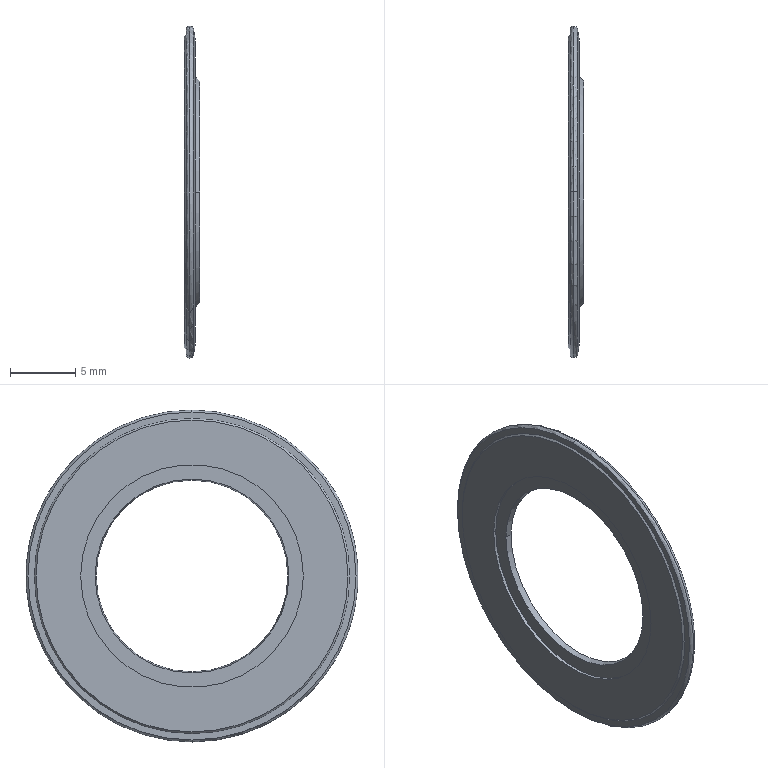Part | SolidWorks | features BaseBody 1 | 1 solid | 23 faces | box 1.155 x 25.353 x 25.353 mm | volume 179.548 mm3 | cone 8 | cylinder 6 | plane 5 | torus 4 | commonest cylinder face diameters 17 x4 23.324 x2
STEP:
#1=CARTESIAN_POINT('',(0.456,0.,12.676));
#2=VERTEX_POINT('',#1);
#3=CARTESIAN_POINT('',(0.456,0.,-12.676));
#4=VERTEX_POINT('',#3);
#5=CARTESIAN_POINT('',(0.456,0.,0.));
#6=DIRECTION('',(1.,0.,0.));
#7=DIRECTION('',(0.,0.,-1.));
#8=AXIS2_PLACEMENT_3D('',#5,#6,#7);
#9=CIRCLE('',#8,12.676);
#10=EDGE_CURVE('',#2,#4,#9,.T.);
#11=ORIENTED_EDGE('',*,*,#10,.T.);
#12=CARTESIAN_POINT('',(0.7554,0.,-12.425));
#13=VERTEX_POINT('',#12);
#14=CARTESIAN_POINT('',(0.456,0.,-12.372));
#15=DIRECTION('',(0.,-1.,0.));
#16=DIRECTION('',(0.,0.,-1.));
#17=AXIS2_PLACEMENT_3D('',#14,#15,#16);
#18=CIRCLE('',#17,0.304);
#19=EDGE_CURVE('',#4,#13,#18,.T.);
#20=ORIENTED_EDGE('',*,*,#19,.T.);
#21=CARTESIAN_POINT('',(0.7554,-12.425,0.));
#22=VERTEX_POINT('',#21);
#23=CARTESIAN_POINT('',(0.7554,0.,0.));
#24=DIRECTION('',(1.,0.,0.));
#25=DIRECTION('',(0.,1.,0.));
#26=AXIS2_PLACEMENT_3D('',#23,#24,#25);
#27=CIRCLE('',#26,12.425);
#28=EDGE_CURVE('',#22,#13,#27,.T.);
#29=ORIENTED_EDGE('',*,*,#28,.F.);
#30=CARTESIAN_POINT('',(0.7554,0.,12.425));
#31=VERTEX_POINT('',#30);
#32=CARTESIAN_POINT('',(0.7554,0.,0.));
#33=DIRECTION('',(1.,0.,0.));
#34=DIRECTION('',(0.,1.,0.));
#35=AXIS2_PLACEMENT_3D('',#32,#33,#34);
#36=CIRCLE('',#35,12.425);
#37=EDGE_CURVE('',#31,#22,#36,.T.);
#38=ORIENTED_EDGE('',*,*,#37,.F.);
#39=CARTESIAN_POINT('',(0.456,0.,12.372));
#40=DIRECTION('',(0.,-1.,0.));
#41=DIRECTION('',(0.,0.,1.));
#42=AXIS2_PLACEMENT_3D('',#39,#40,#41);
#43=CIRCLE('',#42,0.304);
#44=EDGE_CURVE('',#31,#2,#43,.T.);
#45=ORIENTED_EDGE('',*,*,#44,.T.);
#46=EDGE_LOOP('',(#11,#20,#29,#38,#45));
#47=FACE_OUTER_BOUND('',#46,.T.);
#48=CARTESIAN_POINT('',(0.456,0.,0.));
#49=DIRECTION('',(1.,0.,0.));
#50=DIRECTION('',(0.,0.,-1.));
#51=AXIS2_PLACEMENT_3D('',#48,#49,#50);
#52=TOROIDAL_SURFACE('',#51,12.372,0.304);
#53=ADVANCED_FACE('',(#47),#52,.T.);
#54=CARTESIAN_POINT('',(0.1927,12.038,0.));
#55=VERTEX_POINT('',#54);
#56=CARTESIAN_POINT('',(0.1927,-12.038,0.));
#57=VERTEX_POINT('',#56);
#58=CARTESIAN_POINT('',(0.1927,0.,0.));
#59=DIRECTION('',(1.,0.,0.));
#60=DIRECTION('',(0.,1.,0.));
#61=AXIS2_PLACEMENT_3D('',#58,#59,#60);
#62=CIRCLE('',#61,12.038);
#63=EDGE_CURVE('',#55,#57,#62,.T.);
#64=ORIENTED_EDGE('',*,*,#63,.T.);
#65=CARTESIAN_POINT('',(0.1927,0.,0.));
#66=DIRECTION('',(1.,0.,0.));
#67=DIRECTION('',(0.,1.,0.));
#68=AXIS2_PLACEMENT_3D('',#65,#66,#67);
#69=CIRCLE('',#68,12.038);
#70=EDGE_CURVE('',#57,#55,#69,.T.);
#71=ORIENTED_EDGE('',*,*,#70,.T.);
#72=EDGE_LOOP('',(#64,#71));
#73=FACE_BOUND('',#72,.T.);
#74=CARTESIAN_POINT('',(0.1927,0.,-12.524));
#75=VERTEX_POINT('',#74);
#76=CARTESIAN_POINT('',(0.1927,0.,12.524));
#77=VERTEX_POINT('',#76);
#78=CARTESIAN_POINT('',(0.1927,0.,0.));
#79=DIRECTION('',(1.,0.,0.));
#80=DIRECTION('',(0.,1.,0.));
#81=AXIS2_PLACEMENT_3D('',#78,#79,#80);
#82=CIRCLE('',#81,12.524);
#83=EDGE_CURVE('',#75,#77,#82,.T.);
#84=ORIENTED_EDGE('',*,*,#83,.F.);
#85=CARTESIAN_POINT('',(0.1927,0.,0.));
#86=DIRECTION('',(1.,0.,0.));
#87=DIRECTION('',(0.,1.,0.));
#88=AXIS2_PLACEMENT_3D('',#85,#86,#87);
#89=CIRCLE('',#88,12.524);
#90=EDGE_CURVE('',#77,#75,#89,.T.);
#91=ORIENTED_EDGE('',*,*,#90,.F.);
#92=EDGE_LOOP('',(#84,#91));
#93=FACE_OUTER_BOUND('',#92,.T.);
#94=CARTESIAN_POINT('',(0.1927,12.281,0.));
#95=DIRECTION('',(-1.,0.,0.));
#96=DIRECTION('',(0.,1.,0.));
#97=AXIS2_PLACEMENT_3D('',#94,#95,#96);
#98=PLANE('',#97);
#99=ADVANCED_FACE('',(#73,#93),#98,.T.);
#100=CARTESIAN_POINT('',(0.0608,11.906,0.));
#101=VERTEX_POINT('',#100);
#102=CARTESIAN_POINT('',(0.1268,11.972,0.));
#103=DIRECTION('',(0.7071,0.7071,0.));
#104=VECTOR('',#103,1000.);
#105=LINE('',#102,#104);
#106=EDGE_CURVE('',#101,#55,#105,.T.);
#107=ORIENTED_EDGE('',*,*,#106,.T.);
#108=ORIENTED_EDGE('',*,*,#70,.F.);
#109=CARTESIAN_POINT('',(0.0608,-11.906,0.));
#110=VERTEX_POINT('',#109);
#111=CARTESIAN_POINT('',(0.1268,-11.972,0.));
#112=DIRECTION('',(-0.7071,0.7071,0.));
#113=VECTOR('',#112,1000.);
#114=LINE('',#111,#113);
#115=EDGE_CURVE('',#57,#110,#114,.T.);
#116=ORIENTED_EDGE('',*,*,#115,.T.);
#117=CARTESIAN_POINT('',(0.0608,0.,0.));
#118=DIRECTION('',(1.,0.,0.));
#119=DIRECTION('',(0.,1.,0.));
#120=AXIS2_PLACEMENT_3D('',#117,#118,#119);
#121=CIRCLE('',#120,11.906);
#122=EDGE_CURVE('',#110,#101,#121,.T.);
#123=ORIENTED_EDGE('',*,*,#122,.T.);
#124=EDGE_LOOP('',(#107,#108,#116,#123));
#125=FACE_OUTER_BOUND('',#124,.T.);
#126=CARTESIAN_POINT('',(0.1268,0.,0.));
#127=DIRECTION('',(1.,0.,0.));
#128=DIRECTION('',(0.,1.,0.));
#129=AXIS2_PLACEMENT_3D('',#126,#127,#128);
#130=CONICAL_SURFACE('',#129,11.972,0.7854);
#131=ADVANCED_FACE('',(#125),#130,.T.);
#132=CARTESIAN_POINT('',(0.0608,8.5,0.));
#133=VERTEX_POINT('',#132);
#134=CARTESIAN_POINT('',(0.0608,-8.5,0.));
#135=VERTEX_POINT('',#134);
#136=CARTESIAN_POINT('',(0.0608,0.,0.));
#137=DIRECTION('',(1.,0.,0.));
#138=DIRECTION('',(0.,1.,0.));
#139=AXIS2_PLACEMENT_3D('',#136,#137,#138);
#140=CIRCLE('',#139,8.5);
#141=EDGE_CURVE('',#133,#135,#140,.T.);
#142=ORIENTED_EDGE('',*,*,#141,.T.);
#143=CARTESIAN_POINT('',(0.0608,0.,0.));
#144=DIRECTION('',(1.,0.,0.));
#145=DIRECTION('',(0.,1.,0.));
#146=AXIS2_PLACEMENT_3D('',#143,#144,#145);
#147=CIRCLE('',#146,8.5);
#148=EDGE_CURVE('',#135,#133,#147,.T.);
#149=ORIENTED_EDGE('',*,*,#148,.T.);
#150=EDGE_LOOP('',(#142,#149));
#151=FACE_BOUND('',#150,.T.);
#152=CARTESIAN_POINT('',(0.0608,0.,0.));
#153=DIRECTION('',(1.,0.,0.));
#154=DIRECTION('',(0.,1.,0.));
#155=AXIS2_PLACEMENT_3D('',#152,#153,#154);
#156=CIRCLE('',#155,11.906);
#157=EDGE_CURVE('',#101,#110,#156,.T.);
#158=ORIENTED_EDGE('',*,*,#157,.F.);
#159=ORIENTED_EDGE('',*,*,#122,.F.);
#160=EDGE_LOOP('',(#158,#159));
#161=FACE_OUTER_BOUND('',#160,.T.);
#162=CARTESIAN_POINT('',(0.0608,10.203,0.));
#163=DIRECTION('',(-1.,0.,0.));
#164=DIRECTION('',(0.,0.,1.));
#165=AXIS2_PLACEMENT_3D('',#162,#163,#164);
#166=PLANE('',#165);
#167=ADVANCED_FACE('',(#151,#161),#166,.T.);
#168=CARTESIAN_POINT('',(0.2888,8.5,0.));
#169=VERTEX_POINT('',#168);
#170=CARTESIAN_POINT('',(0.1748,8.5,0.));
#171=DIRECTION('',(1.,0.,0.));
#172=VECTOR('',#171,1000.);
#173=LINE('',#170,#172);
#174=EDGE_CURVE('',#133,#169,#173,.T.);
#175=ORIENTED_EDGE('',*,*,#174,.T.);
#176=CARTESIAN_POINT('',(0.2888,-8.5,0.));
#177=VERTEX_POINT('',#176);
#178=CARTESIAN_POINT('',(0.2888,0.,0.));
#179=DIRECTION('',(1.,0.,0.));
#180=DIRECTION('',(0.,1.,0.));
#181=AXIS2_PLACEMENT_3D('',#178,#179,#180);
#182=CIRCLE('',#181,8.5);
#183=EDGE_CURVE('',#169,#177,#182,.T.);
#184=ORIENTED_EDGE('',*,*,#183,.T.);
#185=CARTESIAN_POINT('',(0.1748,-8.5,0.));
#186=DIRECTION('',(-1.,0.,0.));
#187=VECTOR('',#186,1000.);
#188=LINE('',#185,#187);
#189=EDGE_CURVE('',#177,#135,#188,.T.);
#190=ORIENTED_EDGE('',*,*,#189,.T.);
#191=ORIENTED_EDGE('',*,*,#141,.F.);
#192=EDGE_LOOP('',(#175,#184,#190,#191));
#193=FACE_OUTER_BOUND('',#192,.T.);
#194=CARTESIAN_POINT('',(0.1748,0.,0.));
#195=DIRECTION('',(1.,0.,0.));
#196=DIRECTION('',(0.,1.,0.));
#197=AXIS2_PLACEMENT_3D('',#194,#195,#196);
#198=CYLINDRICAL_SURFACE('',#197,8.5);
#199=ADVANCED_FACE('',(#193),#198,.F.);
#200=CARTESIAN_POINT('',(0.2888,7.405,0.));
#201=VERTEX_POINT('',#200);
#202=CARTESIAN_POINT('',(0.2888,-7.405,0.));
#203=VERTEX_POINT('',#202);
#204=CARTESIAN_POINT('',(0.2888,0.,0.));
#205=DIRECTION('',(1.,0.,0.));
#206=DIRECTION('',(0.,1.,0.));
#207=AXIS2_PLACEMENT_3D('',#204,#205,#206);
#208=CIRCLE('',#207,7.405);
#209=EDGE_CURVE('',#201,#203,#208,.T.);
#210=ORIENTED_EDGE('',*,*,#209,.T.);
#211=CARTESIAN_POINT('',(0.2888,0.,0.));
#212=DIRECTION('',(1.,0.,0.));
#213=DIRECTION('',(0.,1.,0.));
#214=AXIS2_PLACEMENT_3D('',#211,#212,#213);
#215=CIRCLE('',#214,7.405);
#216=EDGE_CURVE('',#203,#201,#215,.T.);
#217=ORIENTED_EDGE('',*,*,#216,.T.);
#218=EDGE_LOOP('',(#210,#217));
#219=FACE_BOUND('',#218,.T.);
#220=ORIENTED_EDGE('',*,*,#183,.F.);
#221=CARTESIAN_POINT('',(0.2888,0.,0.));
#222=DIRECTION('',(1.,0.,0.));
#223=DIRECTION('',(0.,1.,0.));
#224=AXIS2_PLACEMENT_3D('',#221,#222,#223);
#225=CIRCLE('',#224,8.5);
#226=EDGE_CURVE('',#177,#169,#225,.T.);
#227=ORIENTED_EDGE('',*,*,#226,.F.);
#228=EDGE_LOOP('',(#220,#227));
#229=FACE_OUTER_BOUND('',#228,.T.);
#230=CARTESIAN_POINT('',(0.2888,7.953,0.));
#231=DIRECTION('',(-1.,0.,0.));
#232=DIRECTION('',(0.,1.,0.));
#233=AXIS2_PLACEMENT_3D('',#230,#231,#232);
#234=PLANE('',#233);
#235=ADVANCED_FACE('',(#219,#229),#234,.T.);
#236=CARTESIAN_POINT('',(0.76,7.322,0.));
#237=VERTEX_POINT('',#236);
#238=CARTESIAN_POINT('',(0.5244,7.364,0.));
#239=DIRECTION('',(0.9848,-0.1736,0.));
#240=VECTOR('',#239,1000.);
#241=LINE('',#238,#240);
#242=EDGE_CURVE('',#201,#237,#241,.T.);
#243=ORIENTED_EDGE('',*,*,#242,.T.);
#244=CARTESIAN_POINT('',(0.76,-7.322,0.));
#245=VERTEX_POINT('',#244);
#246=CARTESIAN_POINT('',(0.76,0.,0.));
#247=DIRECTION('',(1.,0.,0.));
#248=DIRECTION('',(0.,1.,0.));
#249=AXIS2_PLACEMENT_3D('',#246,#247,#248);
#250=CIRCLE('',#249,7.322);
#251=EDGE_CURVE('',#237,#245,#250,.T.);
#252=ORIENTED_EDGE('',*,*,#251,.T.);
#253=CARTESIAN_POINT('',(0.5244,-7.364,0.));
#254=DIRECTION('',(-0.9848,-0.1736,0.));
#255=VECTOR('',#254,1000.);
#256=LINE('',#253,#255);
#257=EDGE_CURVE('',#245,#203,#256,.T.);
#258=ORIENTED_EDGE('',*,*,#257,.T.);
#259=ORIENTED_EDGE('',*,*,#209,.F.);
#260=EDGE_LOOP('',(#243,#252,#258,#259));
#261=FACE_OUTER_BOUND('',#260,.T.);
#262=CARTESIAN_POINT('',(0.5244,0.,0.));
#263=DIRECTION('',(-1.,0.,0.));
#264=DIRECTION('',(0.,1.,0.));
#265=AXIS2_PLACEMENT_3D('',#262,#263,#264);
#266=CONICAL_SURFACE('',#265,7.364,0.1745);
#267=ADVANCED_FACE('',(#261),#266,.F.);
#268=ORIENTED_EDGE('',*,*,#251,.F.);
#269=CARTESIAN_POINT('',(0.76,0.,0.));
#270=DIRECTION('',(1.,0.,0.));
#271=DIRECTION('',(0.,1.,0.));
#272=AXIS2_PLACEMENT_3D('',#269,#270,#271);
#273=CIRCLE('',#272,7.322);
#274=EDGE_CURVE('',#245,#237,#273,.T.);
#275=ORIENTED_EDGE('',*,*,#274,.F.);
#276=EDGE_LOOP('',(#268,#275));
#277=FACE_BOUND('',#276,.T.);
#278=CARTESIAN_POINT('',(0.76,8.5,0.));
#279=VERTEX_POINT('',#278);
#280=CARTESIAN_POINT('',(0.76,-8.5,0.));
#281=VERTEX_POINT('',#280);
#282=CARTESIAN_POINT('',(0.76,0.,0.));
#283=DIRECTION('',(1.,0.,0.));
#284=DIRECTION('',(0.,1.,0.));
#285=AXIS2_PLACEMENT_3D('',#282,#283,#284);
#286=CIRCLE('',#285,8.5);
#287=EDGE_CURVE('',#279,#281,#286,.T.);
#288=ORIENTED_EDGE('',*,*,#287,.T.);
#289=CARTESIAN_POINT('',(0.76,0.,0.));
#290=DIRECTION('',(1.,0.,0.));
#291=DIRECTION('',(0.,1.,0.));
#292=AXIS2_PLACEMENT_3D('',#289,#290,#291);
#293=CIRCLE('',#292,8.5);
#294=EDGE_CURVE('',#281,#279,#293,.T.);
#295=ORIENTED_EDGE('',*,*,#294,.T.);
#296=EDGE_LOOP('',(#288,#295));
#297=FACE_OUTER_BOUND('',#296,.T.);
#298=CARTESIAN_POINT('',(0.76,7.911,0.));
#299=DIRECTION('',(1.,0.,0.));
#300=DIRECTION('',(0.,1.,0.));
#301=AXIS2_PLACEMENT_3D('',#298,#299,#300);
#302=PLANE('',#301);
#303=ADVANCED_FACE('',(#277,#297),#302,.T.);
#304=CARTESIAN_POINT('',(1.216,8.5,0.));
#305=VERTEX_POINT('',#304);
#306=CARTESIAN_POINT('',(0.988,8.5,0.));
#307=DIRECTION('',(1.,0.,0.));
#308=VECTOR('',#307,1000.);
#309=LINE('',#306,#308);
#310=EDGE_CURVE('',#279,#305,#309,.T.);
#311=ORIENTED_EDGE('',*,*,#310,.T.);
#312=CARTESIAN_POINT('',(1.216,-8.5,0.));
#313=VERTEX_POINT('',#312);
#314=CARTESIAN_POINT('',(1.216,0.,0.));
#315=DIRECTION('',(1.,0.,0.));
#316=DIRECTION('',(0.,1.,0.));
#317=AXIS2_PLACEMENT_3D('',#314,#315,#316);
#318=CIRCLE('',#317,8.5);
#319=EDGE_CURVE('',#305,#313,#318,.T.);
#320=ORIENTED_EDGE('',*,*,#319,.T.);
#321=CARTESIAN_POINT('',(0.988,-8.5,0.));
#322=DIRECTION('',(-1.,0.,0.));
#323=VECTOR('',#322,1000.);
#324=LINE('',#321,#323);
#325=EDGE_CURVE('',#313,#281,#324,.T.);
#326=ORIENTED_EDGE('',*,*,#325,.T.);
#327=ORIENTED_EDGE('',*,*,#287,.F.);
#328=EDGE_LOOP('',(#311,#320,#326,#327));
#329=FACE_OUTER_BOUND('',#328,.T.);
#330=CARTESIAN_POINT('',(0.988,0.,0.));
#331=DIRECTION('',(1.,0.,0.));
#332=DIRECTION('',(0.,1.,0.));
#333=AXIS2_PLACEMENT_3D('',#330,#331,#332);
#334=CYLINDRICAL_SURFACE('',#333,8.5);
#335=ADVANCED_FACE('',(#329),#334,.F.);
#336=CARTESIAN_POINT('',(0.5168,9.199,0.));
#337=VERTEX_POINT('',#336);
#338=CARTESIAN_POINT('',(0.8664,8.85,0.));
#339=DIRECTION('',(0.7071,-0.7071,0.));
#340=VECTOR('',#339,1000.);
#341=LINE('',#338,#340);
#342=EDGE_CURVE('',#337,#305,#341,.T.);
#343=ORIENTED_EDGE('',*,*,#342,.T.);
#344=CARTESIAN_POINT('',(1.216,0.,0.));
#345=DIRECTION('',(1.,0.,0.));
#346=DIRECTION('',(0.,1.,0.));
#347=AXIS2_PLACEMENT_3D('',#344,#345,#346);
#348=CIRCLE('',#347,8.5);
#349=EDGE_CURVE('',#313,#305,#348,.T.);
#350=ORIENTED_EDGE('',*,*,#349,.F.);
#351=CARTESIAN_POINT('',(0.5168,-9.199,0.));
#352=VERTEX_POINT('',#351);
#353=CARTESIAN_POINT('',(0.8664,-8.85,0.));
#354=DIRECTION('',(-0.7071,-0.7071,0.));
#355=VECTOR('',#354,1000.);
#356=LINE('',#353,#355);
#357=EDGE_CURVE('',#313,#352,#356,.T.);
#358=ORIENTED_EDGE('',*,*,#357,.T.);
#359=CARTESIAN_POINT('',(0.5168,0.,0.));
#360=DIRECTION('',(1.,0.,0.));
#361=DIRECTION('',(0.,1.,0.));
#362=AXIS2_PLACEMENT_3D('',#359,#360,#361);
#363=CIRCLE('',#362,9.199);
#364=EDGE_CURVE('',#352,#337,#363,.T.);
#365=ORIENTED_EDGE('',*,*,#364,.T.);
#366=EDGE_LOOP('',(#343,#350,#358,#365));
#367=FACE_OUTER_BOUND('',#366,.T.);
#368=CARTESIAN_POINT('',(0.8664,0.,0.));
#369=DIRECTION('',(-1.,0.,0.));
#370=DIRECTION('',(0.,1.,0.));
#371=AXIS2_PLACEMENT_3D('',#368,#369,#370);
#372=CONICAL_SURFACE('',#371,8.85,0.7854);
#373=ADVANCED_FACE('',(#367),#372,.T.);
#374=CARTESIAN_POINT('',(0.5168,0.,0.));
#375=DIRECTION('',(1.,0.,0.));
#376=DIRECTION('',(0.,1.,0.));
#377=AXIS2_PLACEMENT_3D('',#374,#375,#376);
#378=CIRCLE('',#377,9.199);
#379=EDGE_CURVE('',#337,#352,#378,.T.);
#380=ORIENTED_EDGE('',*,*,#379,.F.);
#381=ORIENTED_EDGE('',*,*,#364,.F.);
#382=EDGE_LOOP('',(#380,#381));
#383=FACE_BOUND('',#382,.T.);
#384=CARTESIAN_POINT('',(0.5168,11.662,0.));
#385=VERTEX_POINT('',#384);
#386=CARTESIAN_POINT('',(0.5168,-11.662,0.));
#387=VERTEX_POINT('',#386);
#388=CARTESIAN_POINT('',(0.5168,0.,0.));
#389=DIRECTION('',(1.,0.,0.));
#390=DIRECTION('',(0.,1.,0.));
#391=AXIS2_PLACEMENT_3D('',#388,#389,#390);
#392=CIRCLE('',#391,11.662);
#393=EDGE_CURVE('',#385,#387,#392,.T.);
#394=ORIENTED_EDGE('',*,*,#393,.T.);
#395=CARTESIAN_POINT('',(0.5168,0.,0.));
#396=DIRECTION('',(1.,0.,0.));
#397=DIRECTION('',(0.,1.,0.));
#398=AXIS2_PLACEMENT_3D('',#395,#396,#397);
#399=CIRCLE('',#398,11.662);
#400=EDGE_CURVE('',#387,#385,#399,.T.);
#401=ORIENTED_EDGE('',*,*,#400,.T.);
#402=EDGE_LOOP('',(#394,#401));
#403=FACE_OUTER_BOUND('',#402,.T.);
#404=CARTESIAN_POINT('',(0.5168,10.431,0.));
#405=DIRECTION('',(1.,0.,0.));
#406=DIRECTION('',(0.,1.,0.));
#407=AXIS2_PLACEMENT_3D('',#404,#405,#406);
#408=PLANE('',#407);
#409=ADVANCED_FACE('',(#383,#403),#408,.T.);
#410=CARTESIAN_POINT('',(0.8899,11.662,0.));
#411=VERTEX_POINT('',#410);
#412=CARTESIAN_POINT('',(0.7034,11.662,0.));
#413=DIRECTION('',(1.,0.,0.));
#414=VECTOR('',#413,1000.);
#415=LINE('',#412,#414);
#416=EDGE_CURVE('',#385,#411,#415,.T.);
#417=ORIENTED_EDGE('',*,*,#416,.T.);
#418=CARTESIAN_POINT('',(0.8899,-11.662,0.));
#419=VERTEX_POINT('',#418);
#420=CARTESIAN_POINT('',(0.8899,0.,0.));
#421=DIRECTION('',(1.,0.,0.));
#422=DIRECTION('',(0.,1.,0.));
#423=AXIS2_PLACEMENT_3D('',#420,#421,#422);
#424=CIRCLE('',#423,11.662);
#425=EDGE_CURVE('',#411,#419,#424,.T.);
#426=ORIENTED_EDGE('',*,*,#425,.T.);
#427=CARTESIAN_POINT('',(0.7034,-11.662,0.));
#428=DIRECTION('',(-1.,0.,0.));
#429=VECTOR('',#428,1000.);
#430=LINE('',#427,#429);
#431=EDGE_CURVE('',#419,#387,#430,.T.);
#432=ORIENTED_EDGE('',*,*,#431,.T.);
#433=ORIENTED_EDGE('',*,*,#393,.F.);
#434=EDGE_LOOP('',(#417,#426,#432,#433));
#435=FACE_OUTER_BOUND('',#434,.T.);
#436=CARTESIAN_POINT('',(0.7034,0.,0.));
#437=DIRECTION('',(1.,0.,0.));
#438=DIRECTION('',(0.,1.,0.));
#439=AXIS2_PLACEMENT_3D('',#436,#437,#438);
#440=CYLINDRICAL_SURFACE('',#439,11.662);
#441=ADVANCED_FACE('',(#435),#440,.F.);
#442=CARTESIAN_POINT('',(0.7554,12.425,0.));
#443=VERTEX_POINT('',#442);
#444=CARTESIAN_POINT('',(0.8227,12.044,0.));
#445=DIRECTION('',(0.1736,-0.9848,0.));
#446=VECTOR('',#445,1000.);
#447=LINE('',#444,#446);
#448=EDGE_CURVE('',#443,#411,#447,.T.);
#449=ORIENTED_EDGE('',*,*,#448,.T.);
#450=CARTESIAN_POINT('',(0.8899,0.,0.));
#451=DIRECTION('',(1.,0.,0.));
#452=DIRECTION('',(0.,1.,0.));
#453=AXIS2_PLACEMENT_3D('',#450,#451,#452);
#454=CIRCLE('',#453,11.662);
#455=EDGE_CURVE('',#419,#411,#454,.T.);
#456=ORIENTED_EDGE('',*,*,#455,.F.);
#457=CARTESIAN_POINT('',(0.8227,-12.044,0.));
#458=DIRECTION('',(-0.1736,-0.9848,0.));
#459=VECTOR('',#458,1000.);
#460=LINE('',#457,#459);
#461=EDGE_CURVE('',#419,#22,#460,.T.);
#462=ORIENTED_EDGE('',*,*,#461,.T.);
#463=ORIENTED_EDGE('',*,*,#28,.T.);
#464=CARTESIAN_POINT('',(0.7554,0.,0.));
#465=DIRECTION('',(1.,0.,0.));
#466=DIRECTION('',(0.,1.,0.));
#467=AXIS2_PLACEMENT_3D('',#464,#465,#466);
#468=CIRCLE('',#467,12.425);
#469=EDGE_CURVE('',#13,#443,#468,.T.);
#470=ORIENTED_EDGE('',*,*,#469,.T.);
#471=EDGE_LOOP('',(#449,#456,#462,#463,#470));
#472=FACE_OUTER_BOUND('',#471,.T.);
#473=CARTESIAN_POINT('',(0.8227,0.,0.));
#474=DIRECTION('',(-1.,0.,0.));
#475=DIRECTION('',(0.,1.,0.));
#476=AXIS2_PLACEMENT_3D('',#473,#474,#475);
#477=CONICAL_SURFACE('',#476,12.044,1.396);
#478=ADVANCED_FACE('',(#472),#477,.T.);
#479=ORIENTED_EDGE('',*,*,#448,.F.);
#480=CARTESIAN_POINT('',(0.7554,0.,0.));
#481=DIRECTION('',(1.,0.,0.));
#482=DIRECTION('',(0.,1.,0.));
#483=AXIS2_PLACEMENT_3D('',#480,#481,#482);
#484=CIRCLE('',#483,12.425);
#485=EDGE_CURVE('',#443,#31,#484,.T.);
#486=ORIENTED_EDGE('',*,*,#485,.T.);
#487=ORIENTED_EDGE('',*,*,#37,.T.);
#488=ORIENTED_EDGE('',*,*,#461,.F.);
#489=ORIENTED_EDGE('',*,*,#425,.F.);
#490=EDGE_LOOP('',(#479,#486,#487,#488,#489));
#491=FACE_OUTER_BOUND('',#490,.T.);
#492=CARTESIAN_POINT('',(0.8227,0.,0.));
#493=DIRECTION('',(-1.,0.,0.));
#494=DIRECTION('',(0.,1.,0.));
#495=AXIS2_PLACEMENT_3D('',#492,#493,#494);
#496=CONICAL_SURFACE('',#495,12.044,1.396);
#497=ADVANCED_FACE('',(#491),#496,.T.);
#498=ORIENTED_EDGE('',*,*,#416,.F.);
#499=ORIENTED_EDGE('',*,*,#400,.F.);
#500=ORIENTED_EDGE('',*,*,#431,.F.);
#501=ORIENTED_EDGE('',*,*,#455,.T.);
#502=EDGE_LOOP('',(#498,#499,#500,#501));
#503=FACE_OUTER_BOUND('',#502,.T.);
#504=CARTESIAN_POINT('',(0.7034,0.,0.));
#505=DIRECTION('',(1.,0.,0.));
#506=DIRECTION('',(0.,1.,0.));
#507=AXIS2_PLACEMENT_3D('',#504,#505,#506);
#508=CYLINDRICAL_SURFACE('',#507,11.662);
#509=ADVANCED_FACE('',(#503),#508,.F.);
#510=ORIENTED_EDGE('',*,*,#342,.F.);
#511=ORIENTED_EDGE('',*,*,#379,.T.);
#512=ORIENTED_EDGE('',*,*,#357,.F.);
#513=ORIENTED_EDGE('',*,*,#319,.F.);
#514=EDGE_LOOP('',(#510,#511,#512,#513));
#515=FACE_OUTER_BOUND('',#514,.T.);
#516=CARTESIAN_POINT('',(0.8664,0.,0.));
#517=DIRECTION('',(-1.,0.,0.));
#518=DIRECTION('',(0.,1.,0.));
#519=AXIS2_PLACEMENT_3D('',#516,#517,#518);
#520=CONICAL_SURFACE('',#519,8.85,0.7854);
#521=ADVANCED_FACE('',(#515),#520,.T.);
#522=ORIENTED_EDGE('',*,*,#310,.F.);
#523=ORIENTED_EDGE('',*,*,#294,.F.);
#524=ORIENTED_EDGE('',*,*,#325,.F.);
#525=ORIENTED_EDGE('',*,*,#349,.T.);
#526=EDGE_LOOP('',(#522,#523,#524,#525));
#527=FACE_OUTER_BOUND('',#526,.T.);
#528=CARTESIAN_POINT('',(0.988,0.,0.));
#529=DIRECTION('',(1.,0.,0.));
#530=DIRECTION('',(0.,1.,0.));
#531=AXIS2_PLACEMENT_3D('',#528,#529,#530);
#532=CYLINDRICAL_SURFACE('',#531,8.5);
#533=ADVANCED_FACE('',(#527),#532,.F.);
#534=ORIENTED_EDGE('',*,*,#242,.F.);
#535=ORIENTED_EDGE('',*,*,#216,.F.);
#536=ORIENTED_EDGE('',*,*,#257,.F.);
#537=ORIENTED_EDGE('',*,*,#274,.T.);
#538=EDGE_LOOP('',(#534,#535,#536,#537));
#539=FACE_OUTER_BOUND('',#538,.T.);
#540=CARTESIAN_POINT('',(0.5244,0.,0.));
#541=DIRECTION('',(-1.,0.,0.));
#542=DIRECTION('',(0.,1.,0.));
#543=AXIS2_PLACEMENT_3D('',#540,#541,#542);
#544=CONICAL_SURFACE('',#543,7.364,0.1745);
#545=ADVANCED_FACE('',(#539),#544,.F.);
#546=ORIENTED_EDGE('',*,*,#174,.F.);
#547=ORIENTED_EDGE('',*,*,#148,.F.);
#548=ORIENTED_EDGE('',*,*,#189,.F.);
#549=ORIENTED_EDGE('',*,*,#226,.T.);
#550=EDGE_LOOP('',(#546,#547,#548,#549));
#551=FACE_OUTER_BOUND('',#550,.T.);
#552=CARTESIAN_POINT('',(0.1748,0.,0.));
#553=DIRECTION('',(1.,0.,0.));
#554=DIRECTION('',(0.,1.,0.));
#555=AXIS2_PLACEMENT_3D('',#552,#553,#554);
#556=CYLINDRICAL_SURFACE('',#555,8.5);
#557=ADVANCED_FACE('',(#551),#556,.F.);
#558=ORIENTED_EDGE('',*,*,#106,.F.);
#559=ORIENTED_EDGE('',*,*,#157,.T.);
#560=ORIENTED_EDGE('',*,*,#115,.F.);
#561=ORIENTED_EDGE('',*,*,#63,.F.);
#562=EDGE_LOOP('',(#558,#559,#560,#561));
#563=FACE_OUTER_BOUND('',#562,.T.);
#564=CARTESIAN_POINT('',(0.1268,0.,0.));
#565=DIRECTION('',(1.,0.,0.));
#566=DIRECTION('',(0.,1.,0.));
#567=AXIS2_PLACEMENT_3D('',#564,#565,#566);
#568=CONICAL_SURFACE('',#567,11.972,0.7854);
#569=ADVANCED_FACE('',(#563),#568,.T.);
#570=CARTESIAN_POINT('',(0.456,0.,0.));
#571=DIRECTION('',(1.,0.,0.));
#572=DIRECTION('',(0.,0.,-1.));
#573=AXIS2_PLACEMENT_3D('',#570,#571,#572);
#574=CIRCLE('',#573,12.676);
#575=EDGE_CURVE('',#4,#2,#574,.T.);
#576=ORIENTED_EDGE('',*,*,#575,.T.);
#577=ORIENTED_EDGE('',*,*,#44,.F.);
#578=ORIENTED_EDGE('',*,*,#485,.F.);
#579=ORIENTED_EDGE('',*,*,#469,.F.);
#580=ORIENTED_EDGE('',*,*,#19,.F.);
#581=EDGE_LOOP('',(#576,#577,#578,#579,#580));
#582=FACE_OUTER_BOUND('',#581,.T.);
#583=CARTESIAN_POINT('',(0.456,0.,0.));
#584=DIRECTION('',(1.,0.,0.));
#585=DIRECTION('',(0.,0.,-1.));
#586=AXIS2_PLACEMENT_3D('',#583,#584,#585);
#587=TOROIDAL_SURFACE('',#586,12.372,0.304);
#588=ADVANCED_FACE('',(#582),#587,.T.);
#589=ORIENTED_EDGE('',*,*,#575,.F.);
#590=CARTESIAN_POINT('',(0.456,0.,-12.372));
#591=DIRECTION('',(0.,-1.,0.));
#592=DIRECTION('',(0.,0.,-1.));
#593=AXIS2_PLACEMENT_3D('',#590,#591,#592);
#594=CIRCLE('',#593,0.304);
#595=EDGE_CURVE('',#75,#4,#594,.T.);
#596=ORIENTED_EDGE('',*,*,#595,.F.);
#597=ORIENTED_EDGE('',*,*,#83,.T.);
#598=CARTESIAN_POINT('',(0.456,0.,12.372));
#599=DIRECTION('',(0.,-1.,0.));
#600=DIRECTION('',(0.,0.,1.));
#601=AXIS2_PLACEMENT_3D('',#598,#599,#600);
#602=CIRCLE('',#601,0.304);
#603=EDGE_CURVE('',#2,#77,#602,.T.);
#604=ORIENTED_EDGE('',*,*,#603,.F.);
#605=EDGE_LOOP('',(#589,#596,#597,#604));
#606=FACE_OUTER_BOUND('',#605,.T.);
#607=CARTESIAN_POINT('',(0.456,0.,0.));
#608=DIRECTION('',(1.,0.,0.));
#609=DIRECTION('',(0.,0.,-1.));
#610=AXIS2_PLACEMENT_3D('',#607,#608,#609);
#611=TOROIDAL_SURFACE('',#610,12.372,0.304);
#612=ADVANCED_FACE('',(#606),#611,.T.);
#613=ORIENTED_EDGE('',*,*,#10,.F.);
#614=ORIENTED_EDGE('',*,*,#603,.T.);
#615=ORIENTED_EDGE('',*,*,#90,.T.);
#616=ORIENTED_EDGE('',*,*,#595,.T.);
#617=EDGE_LOOP('',(#613,#614,#615,#616));
#618=FACE_OUTER_BOUND('',#617,.T.);
#619=CARTESIAN_POINT('',(0.456,0.,0.));
#620=DIRECTION('',(1.,0.,0.));
#621=DIRECTION('',(0.,0.,-1.));
#622=AXIS2_PLACEMENT_3D('',#619,#620,#621);
#623=TOROIDAL_SURFACE('',#622,12.372,0.304);
#624=ADVANCED_FACE('',(#618),#623,.T.);
#625=CLOSED_SHELL('',(#53,#99,#131,#167,#199,#235,#267,#303,#335,#373,#409,#441,#478,#497,#509,#521,#533,#545,#557,#569,#588,#612,#624));
#626=MANIFOLD_SOLID_BREP('',#625);
#627=CARTESIAN_POINT('',(0.,0.,0.));
#628=DIRECTION('',(0.,0.,1.));
#629=DIRECTION('',(1.,0.,0.));
#630=AXIS2_PLACEMENT_3D('',#627,#628,#629);
#631=(LENGTH_UNIT()NAMED_UNIT(*)SI_UNIT(.MILLI.,.METRE.));
#632=UNCERTAINTY_MEASURE_WITH_UNIT(LENGTH_MEASURE(0.00001),#631,'','');
#633=(NAMED_UNIT(*)PLANE_ANGLE_UNIT()SI_UNIT($,.RADIAN.));
#634=(NAMED_UNIT(*)SI_UNIT($,.STERADIAN.)SOLID_ANGLE_UNIT());
#635=(GEOMETRIC_REPRESENTATION_CONTEXT(3)GLOBAL_UNCERTAINTY_ASSIGNED_CONTEXT((#632))GLOBAL_UNIT_ASSIGNED_CONTEXT((#631,#633,#634))REPRESENTATION_CONTEXT('',''));
#636=ADVANCED_BREP_SHAPE_REPRESENTATION('',(#626,#630),#635);